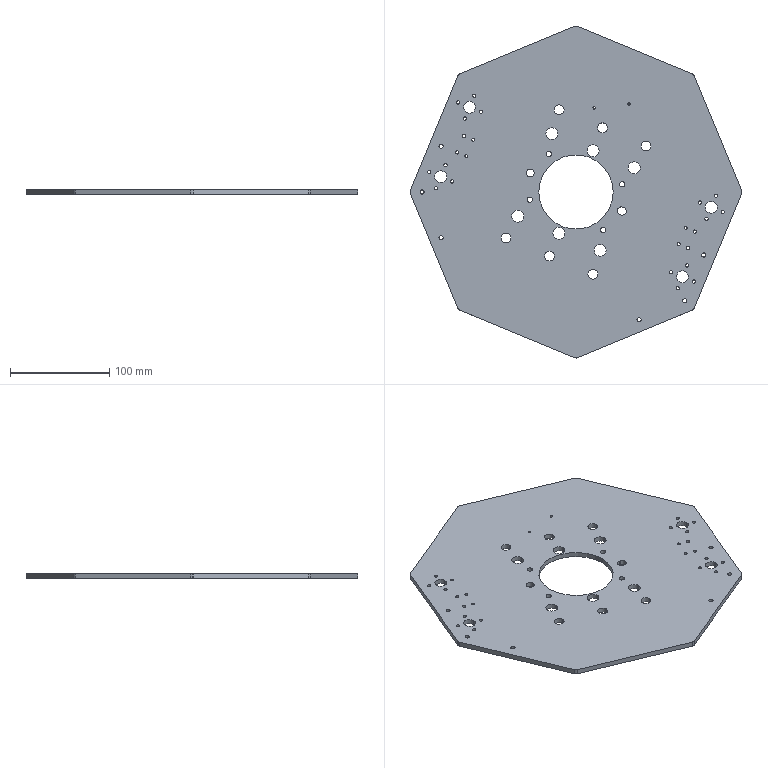Part | SolidWorks | features HoleWzd 5, ICE 5, Cut 4, 3DProfileFeature 2, Extrusion 1, Fillet 1 | 1 solid | 132 faces | box 335.047 x 335.047 x 5 mm | volume 365472 mm3 | cylinder 120 | plane 12 | commonest cylinder face diameters 3.3 x40 12 x20 4.2 x12 10 x12 6 x9 3 x8